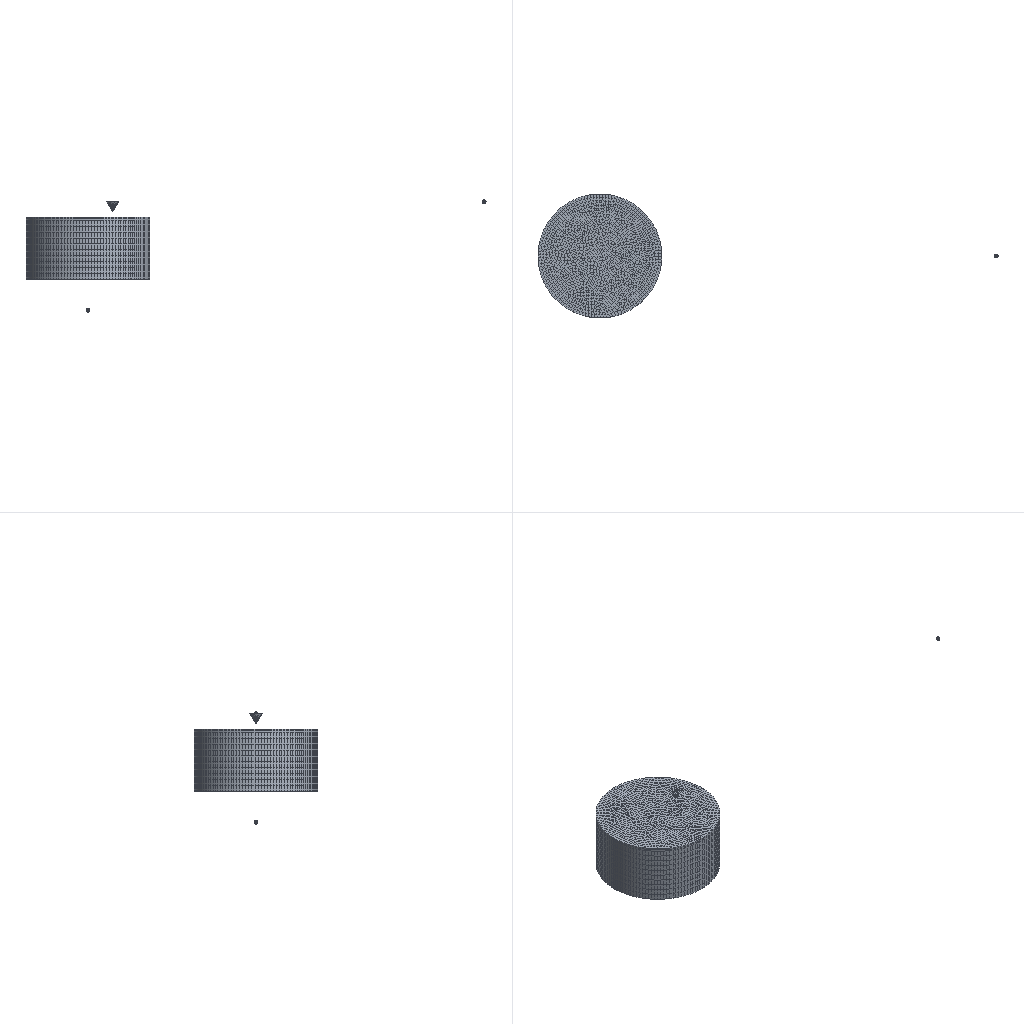Simulation study | abaqus
Set-up summary:
category,name,step,type,value,unit,region
solver,abaqus
solver,version,,,Abaqus/Explicit 2020
units,not stated in the deck,,not stated
analysis,deck,,transient,transient
load_step,Step-1,Step-1,transient
load_step,requested,,,1
mesh,nodes,,,27952
mesh,elements,,,30285
element_type,C3D4,,solid,8198
element_type,C3D8R,,solid,19488
element_type,C3D10M,,solid,2599
load,load commands in deck,,count,2
bc,support commands in deck,,count,7
material,TOOL,,in results
material,WORK,,in results
material,ZHONGJIAN,,in results
check,setup vs results,,match,"per instance, exact: element labels, types and connectivity; labels of the nodes the elements use; coordinates not compared"
Abaqus input file, long lists of numbers shortened:
*Heading
** Job name: Job-1 Model name: Model-1
** Generated by: Abaqus/CAE 2020
*Preprint, echo=NO, model=NO, history=NO, contact=NO
**
** PARTS
**
*Part, name=tool
*Node
      1, 0.07265, -0.0003314,           0.
      2,           0.,           0.,           0.
** (4216 more lines like these left out)
*Element, type=C3D10M
   1,  357,  358,  359,  360,  636,  635,  634,  638,  637,  639
   2,  357,  361,  362,  363,  642,  641,  640,  644,  643,  645
** (2597 more lines like these left out)
*Nset, nset=Set-1, generate
    1,  4218,     1
*Elset, elset=Set-1, generate
    1,  2599,     1
** Section: tool
*Solid Section, elset=Set-1, material=tool
,
*End Part
**
*Part, name=work
*Node
      1,    8.841,  -17.94,          19.
      2,   14.142,  -14.142,           0.
** (21942 more lines like these left out)
*Element, type=C3D8R
    1,    54,   669,   660,    53,  3554,  6614,  6605,  3553
    2,   579,  1605,   918,  1626,  6524,  7550,  6863,  7571
** (19486 more lines like these left out)
*Nset, nset=Set-1, generate
     1,  21944,      1
*Elset, elset=Set-1, generate
     1,  19488,      1
** Section: work
*Solid Section, elset=Set-1, material=work
,
*End Part
**
*Part, name=zhongjian
*Node
      1,  0.1247,  0.5869,           0.
      2,  0.244,  0.5481,           0.
** (892 more lines like these left out)
*Element, type=C3D4
   1, 390, 391, 392, 393
   2, 390, 394, 395, 393
** (4097 more lines like these left out)
*Node
    895,           0., -3.67394056e-17,           0.
*Nset, nset=zhongjian-RefPt_, internal
895,
*Nset, nset=Set-12, generate
   1,  894,    1
*Elset, elset=Set-12, generate
    1,  4099,     1
** Section: zhongjian
*Solid Section, elset=Set-12, material=ZHONGJIAN
,
*End Part
**
**
** ASSEMBLY
**
*Assembly, name=Assembly
**
*Instance, name=tool-1, part=tool
          8.,           0.,          22.
          8.,           0.,          22., 7.,           0.,          22., 90.
*End Instance
**
*Instance, name=work-1, part=work
*End Instance
**
*Instance, name=zhongjian-1, part=zhongjian
        128.,           0.,          25.
*End Instance
**
*Instance, name=zhongjian-2, part=zhongjian
          0.,           0.,         -10.
*End Instance
**
*Node
      1,           0.,           0.,          20.
*Node
      2,           8., -6.12323426e-17,          25.
*Nset, nset=O```
 2,
*Nset, nset=Set-2, instance=work-1
    2,  130,  131,  132,  133,  134,  135,  136,  137,  138,  139,  140,  141,  142,  143,  144
  145,  146,  147,  148,  149,  150,  151,  152,  153,  154,  155,  156,  157,  158,  159,  160
** (104 more lines like these left out)
*Elset, elset=Set-2, instance=work-1, generate
 14617,  16240,      1
*Nset, nset=Set-6, instance=zhongjian-1
 895,
*Nset, nset=Set-11, instance=zhongjian-1
 895,
*Nset, nset=Set-12, instance=zhongjian-1, generate
   1,  389,    1
*Elset, elset=Set-12, instance=zhongjian-1
    4,   92,  207,  218,  228,  238,  271,  289,  299,  351,  358,  363,  392,  402,  418,  434
  457,  464,  525,  530,  587,  619,  629,  652,  671,  724,  817,  883,  901,  938,  980, 1055
** (47 more lines like these left out)
*Nset, nset=Set-14, instance=zhongjian-1
   1,   2,   3,   4,   5,   6,   7,   8,   9,  10,  11,  12,  13,  14,  15,  16
  17,  18,  19,  20,  21,  22,  23,  24,  25,  26,  27,  28,  29,  30,  31,  32
** (23 more lines like these left out)
*Elset, elset=Set-14, instance=zhongjian-1
    4,   92,  207,  218,  228,  238,  271,  289,  299,  351,  358,  363,  392,  402,  418,  434
  457,  464,  525,  530,  587,  619,  629,  652,  671,  724,  817,  883,  901,  938,  980, 1055
** (47 more lines like these left out)
*Nset, nset=Set-15, instance=zhongjian-1
 895,
*Nset, nset=Set-20
 2,
*Nset, nset=Set-21
 2,
*Nset, nset=Set-23, instance=zhongjian-2
 895,
*Nset, nset=Set-24, instance=work-1
    2,  130,  131,  132,  133,  134,  135,  136,  137,  138,  139,  140,  141,  142,  143,  144
  145,  146,  147,  148,  149,  150,  151,  152,  153,  154,  155,  156,  157,  158,  159,  160
** (104 more lines like these left out)
*Elset, elset=Set-24, instance=work-1, generate
 14617,  16240,      1
*Nset, nset=Set-27, instance=zhongjian-1
 895,
*Nset, nset=b_Set-4, instance=tool-1, generate
    1,  4218,     1
*Elset, elset=b_Set-4, instance=tool-1, generate
    1,  2599,     1
*Nset, nset=m_Set-7, instance=zhongjian-1
 895,
*Nset, nset=m_Set-10
 2,
*Nset, nset=m_Set-13, instance=zhongjian-1
 895,
*Nset, nset=m_Set-22, instance=zhongjian-2
 895,
*Nset, nset=m_Set-25, instance=zhongjian-1
 895,
*Nset, nset=m_Set-31, instance=zhongjian-1
 895,
*Nset, nset=s_Set-9, instance=work-1
     1,     3,     4,     5,     6,     7,     8,     9,    10,    11,    12,    13,    14,    15,    16,    17
    18,    19,    20,    21,    22,    23,    24,    25,    26,    27,    28,    29,    30,    31,    32,    33
** (315 more lines like these left out)
*Elset, elset=s_Set-9, instance=work-1, generate
 16241,  19488,      1
*Nset, nset=s_Set-28, instance=zhongjian-1
 895,
*Nset, nset=s_Set-29, instance=zhongjian-1
 895,
*Nset, nset=s_Set-30, instance=zhongjian-1
 15,
*Nset, nset=_PickedSet18, internal
 2,
*Elset, elset=_m_Surf-3_S3, internal, instance=tool-1
   78,   91,   99,  120,  134,  140,  142,  156,  171,  174,  175,  227,  236,  300,  303,  334
  345,  361,  391,  438,  442,  466,  473,  545,  556,  563,  577,  583,  616,  617,  669,  683
** (35 more lines like these left out)
*Elset, elset=_m_Surf-3_S4, internal, instance=tool-1
  110,  555, 1022, 1034, 1139, 1517, 1537, 1685, 1759, 1847, 2324, 2399
*Elset, elset=_m_Surf-3_S1, internal, instance=tool-1
  346,  510,  736,  906,  960,  978, 1446, 1805, 2076, 2161, 2174, 2238, 2314, 2341, 2522
*Elset, elset=_m_Surf-3_S2, internal, instance=tool-1
  665,  757, 1449, 1497, 1588, 1601, 1647, 1705, 1760, 1790, 1821, 1831, 1834, 1878, 1899, 1962
 2052, 2064, 2112, 2437
*Surface, type=ELEMENT, name=m_Surf-3
_m_Surf-3_S3, S3
_m_Surf-3_S4, S4
_m_Surf-3_S2, S2
_m_Surf-3_S1, S1
*Elset, elset=_s_Surf-1_S3, internal, instance=tool-1
   78,   91,   99,  120,  134,  140,  142,  156,  171,  174,  175,  227,  236,  300,  303,  334
  345,  361,  391,  438,  442,  466,  473,  497,  545,  563,  577,  583,  617,  669,  683,  709
** (36 more lines like these left out)
*Elset, elset=_s_Surf-1_S4, internal, instance=tool-1
  110,  555,  583,  848,  887, 1022, 1034, 1139, 1430, 1455, 1469, 1511, 1517, 1537, 1569, 1610
 1638, 1685, 1719, 1847, 1857, 1877, 2324, 2399, 2425, 2508
*Elset, elset=_s_Surf-1_S1, internal, instance=tool-1
  346,  510,  736,  906,  960,  978, 1428, 1429, 1431, 1446, 1527, 1622, 1713, 1715, 1805, 1953
 2076, 2153, 2161, 2174, 2238, 2302, 2341, 2522
*Elset, elset=_s_Surf-1_S2, internal, instance=tool-1
  665,  757, 1164, 1363, 1446, 1449, 1497, 1521, 1574, 1588, 1601, 1634, 1639, 1643, 1646, 1647
 1697, 1705, 1714, 1760, 1762, 1788, 1790, 1821, 1831, 1834, 1878, 1899, 1962, 1970, 1982, 1995
** (1 more lines like these left out)
*Surface, type=ELEMENT, name=s_Surf-1
_s_Surf-1_S3, S3
_s_Surf-1_S4, S4
_s_Surf-1_S2, S2
_s_Surf-1_S1, S1
*Elset, elset=_s_Surf-2_S3, internal, instance=tool-1
   78,   91,   99,  120,  134,  140,  142,  156,  171,  174,  175,  227,  236,  300,  303,  334
  345,  361,  391,  438,  442,  466,  473,  497,  545,  563,  577,  583,  617,  669,  683,  709
** (36 more lines like these left out)
*Elset, elset=_s_Surf-2_S4, internal, instance=tool-1
  110,  555,  583,  848,  887, 1022, 1034, 1139, 1430, 1455, 1469, 1511, 1517, 1537, 1569, 1610
 1638, 1685, 1719, 1847, 1857, 1877, 2324, 2399, 2425, 2508
*Elset, elset=_s_Surf-2_S1, internal, instance=tool-1
  346,  510,  736,  906,  960,  978, 1428, 1429, 1431, 1446, 1527, 1622, 1713, 1715, 1805, 1953
 2076, 2153, 2161, 2174, 2238, 2302, 2341, 2522
*Elset, elset=_s_Surf-2_S2, internal, instance=tool-1
  665,  757, 1164, 1363, 1446, 1449, 1497, 1521, 1574, 1588, 1601, 1634, 1639, 1643, 1646, 1647
 1697, 1705, 1714, 1760, 1762, 1788, 1790, 1821, 1831, 1834, 1878, 1899, 1962, 1970, 1982, 1995
** (1 more lines like these left out)
*Surface, type=ELEMENT, name=s_Surf-2
_s_Surf-2_S3, S3
_s_Surf-2_S4, S4
_s_Surf-2_S2, S2
_s_Surf-2_S1, S1
*Elset, elset=_s_Surf-4_S3, internal, instance=tool-1
   78,   91,   99,  120,  134,  140,  142,  156,  171,  174,  175,  227,  236,  300,  303,  334
  345,  361,  391,  438,  442,  466,  473,  497,  545,  563,  577,  583,  617,  669,  683,  709
** (36 more lines like these left out)
*Elset, elset=_s_Surf-4_S4, internal, instance=tool-1
  110,  555,  583,  848,  887, 1022, 1034, 1139, 1430, 1455, 1469, 1511, 1517, 1537, 1569, 1610
 1638, 1685, 1719, 1847, 1857, 1877, 2324, 2399, 2425, 2508
*Elset, elset=_s_Surf-4_S1, internal, instance=tool-1
  346,  510,  736,  906,  960,  978, 1428, 1429, 1431, 1446, 1527, 1622, 1713, 1715, 1805, 1953
 2076, 2153, 2161, 2174, 2238, 2302, 2341, 2522
*Elset, elset=_s_Surf-4_S2, internal, instance=tool-1
  665,  757, 1164, 1363, 1446, 1449, 1497, 1521, 1574, 1588, 1601, 1634, 1639, 1643, 1646, 1647
 1697, 1705, 1714, 1760, 1762, 1788, 1790, 1821, 1831, 1834, 1878, 1899, 1962, 1970, 1982, 1995
** (1 more lines like these left out)
*Surface, type=ELEMENT, name=s_Surf-4
_s_Surf-4_S3, S3
_s_Surf-4_S4, S4
_s_Surf-4_S2, S2
_s_Surf-4_S1, S1
*Elset, elset=_s_Surf-5_S4, internal, instance=zhongjian-1
    4,  207,  619, 1283, 1533, 1714, 1784, 1867, 1928, 1998, 2148, 2163, 2289, 2383, 2459, 2481
 2483, 2546, 2592, 2733, 2800, 2803, 2851, 2913, 2943, 2958, 3155, 3221, 3281, 3352, 3359, 3364
** (1 more lines like these left out)
*Elset, elset=_s_Surf-5_S3, internal, instance=zhongjian-1
   92,  218,  228,  238,  289,  299,  351,  358,  363,  392,  402,  418,  434,  457,  464,  587
  671,  724,  817,  883,  938,  980, 1058, 1138, 1180, 1244, 1252, 1309, 1325, 1385, 1394, 1402
** (42 more lines like these left out)
*Elset, elset=_s_Surf-5_S1, internal, instance=zhongjian-1
  271,  525,  901, 1055, 1059, 1234, 1942, 2336, 2472, 2613, 2645, 2752, 3469, 3771, 3814
*Elset, elset=_s_Surf-5_S2, internal, instance=zhongjian-1
  530,  629,  652, 1859, 1898, 1899, 1979, 2210, 2256, 2330, 2343, 2370, 2910, 3041, 3271, 3345
 3375, 3392, 3471, 3618, 3844, 3951
*Surface, type=ELEMENT, name=s_Surf-5
_s_Surf-5_S4, S4
_s_Surf-5_S3, S3
_s_Surf-5_S2, S2
_s_Surf-5_S1, S1
*Elset, elset=_s_Surf-6_S3, internal, instance=tool-1
   78,   91,   99,  120,  134,  140,  142,  156,  171,  174,  175,  227,  236,  300,  303,  334
  345,  361,  391,  438,  442,  466,  473,  497,  545,  563,  577,  583,  617,  669,  683,  709
** (36 more lines like these left out)
*Elset, elset=_s_Surf-6_S4, internal, instance=tool-1
  110,  555,  583,  848,  887, 1022, 1034, 1139, 1430, 1455, 1469, 1511, 1517, 1537, 1569, 1610
 1638, 1685, 1719, 1847, 1857, 1877, 2324, 2399, 2425, 2508
*Elset, elset=_s_Surf-6_S1, internal, instance=tool-1
  346,  510,  736,  906,  960,  978, 1428, 1429, 1431, 1446, 1527, 1622, 1713, 1715, 1805, 1953
 2076, 2153, 2161, 2174, 2238, 2302, 2341, 2522
*Elset, elset=_s_Surf-6_S2, internal, instance=tool-1
  665,  757, 1164, 1363, 1446, 1449, 1497, 1521, 1574, 1588, 1601, 1634, 1639, 1643, 1646, 1647
 1697, 1705, 1714, 1760, 1762, 1788, 1790, 1821, 1831, 1834, 1878, 1899, 1962, 1970, 1982, 1995
** (1 more lines like these left out)
*Surface, type=ELEMENT, name=s_Surf-6
_s_Surf-6_S3, S3
_s_Surf-6_S4, S4
_s_Surf-6_S2, S2
_s_Surf-6_S1, S1
*Elset, elset=_s_Surf-7_S4, internal, instance=zhongjian-1
    4,  207,  619, 1283, 1533, 1714, 1784, 1867, 1928, 1998, 2148, 2163, 2289, 2383, 2459, 2481
 2483, 2546, 2592, 2733, 2800, 2803, 2851, 2913, 2943, 2958, 3155, 3221, 3281, 3352, 3359, 3364
** (1 more lines like these left out)
*Elset, elset=_s_Surf-7_S3, internal, instance=zhongjian-1
   92,  218,  228,  238,  289,  299,  351,  358,  363,  392,  402,  418,  434,  457,  464,  587
  671,  724,  817,  883,  938,  980, 1058, 1138, 1180, 1244, 1252, 1309, 1325, 1385, 1394, 1402
** (42 more lines like these left out)
*Elset, elset=_s_Surf-7_S1, internal, instance=zhongjian-1
  271,  525,  901, 1055, 1059, 1234, 1942, 2336, 2472, 2613, 2645, 2752, 3469, 3771, 3814
*Elset, elset=_s_Surf-7_S2, internal, instance=zhongjian-1
  530,  629,  652, 1859, 1898, 1899, 1979, 2210, 2256, 2330, 2343, 2370, 2910, 3041, 3271, 3345
 3375, 3392, 3471, 3618, 3844, 3951
*Surface, type=ELEMENT, name=s_Surf-7
_s_Surf-7_S4, S4
_s_Surf-7_S3, S3
_s_Surf-7_S2, S2
_s_Surf-7_S1, S1
*Elset, elset=_s_Surf-8_S3, internal, instance=tool-1
   78,   91,   99,  120,  134,  140,  142,  156,  171,  174,  175,  227,  236,  300,  303,  334
  345,  361,  391,  438,  442,  466,  473,  497,  545,  563,  577,  583,  617,  669,  683,  709
** (36 more lines like these left out)
*Elset, elset=_s_Surf-8_S4, internal, instance=tool-1
  110,  555,  583,  848,  887, 1022, 1034, 1139, 1430, 1455, 1469, 1511, 1517, 1537, 1569, 1610
 1638, 1685, 1719, 1847, 1857, 1877, 2324, 2399, 2425, 2508
*Elset, elset=_s_Surf-8_S1, internal, instance=tool-1
  346,  510,  736,  906,  960,  978, 1428, 1429, 1431, 1446, 1527, 1622, 1713, 1715, 1805, 1953
 2076, 2153, 2161, 2174, 2238, 2302, 2341, 2522
*Elset, elset=_s_Surf-8_S2, internal, instance=tool-1
  665,  757, 1164, 1363, 1446, 1449, 1497, 1521, 1574, 1588, 1601, 1634, 1639, 1643, 1646, 1647
 1697, 1705, 1714, 1760, 1762, 1788, 1790, 1821, 1831, 1834, 1878, 1899, 1962, 1970, 1982, 1995
** (1 more lines like these left out)
*Surface, type=ELEMENT, name=s_Surf-8
_s_Surf-8_S3, S3
_s_Surf-8_S4, S4
_s_Surf-8_S2, S2
_s_Surf-8_S1, S1
*Elset, elset=_s_Surf-9_S4, internal, instance=zhongjian-1
    4,  207,  619, 1283, 1533, 1714, 1784, 1867, 1928, 1998, 2148, 2163, 2289, 2383, 2459, 2481
 2483, 2546, 2592, 2733, 2800, 2803, 2851, 2913, 2943, 2958, 3155, 3221, 3281, 3352, 3359, 3364
** (1 more lines like these left out)
*Elset, elset=_s_Surf-9_S3, internal, instance=zhongjian-1
   92,  218,  228,  238,  289,  299,  351,  358,  363,  392,  402,  418,  434,  457,  464,  587
  671,  724,  817,  883,  938,  980, 1058, 1138, 1180, 1244, 1252, 1309, 1325, 1385, 1394, 1402
** (42 more lines like these left out)
*Elset, elset=_s_Surf-9_S1, internal, instance=zhongjian-1
  271,  525,  901, 1055, 1059, 1234, 1942, 2336, 2472, 2613, 2645, 2752, 3469, 3771, 3814
*Elset, elset=_s_Surf-9_S2, internal, instance=zhongjian-1
  530,  629,  652, 1859, 1898, 1899, 1979, 2210, 2256, 2330, 2343, 2370, 2910, 3041, 3271, 3345
 3375, 3392, 3471, 3618, 3844, 3951
*Surface, type=ELEMENT, name=s_Surf-9
_s_Surf-9_S4, S4
_s_Surf-9_S3, S3
_s_Surf-9_S2, S2
_s_Surf-9_S1, S1
*Elset, elset=_s_Surf-10_S3, internal, instance=tool-1
   78,   91,   99,  120,  134,  140,  142,  156,  171,  174,  175,  227,  236,  300,  303,  334
  345,  361,  391,  438,  442,  466,  473,  497,  545,  556,  563,  577,  583,  616,  617,  669
** (37 more lines like these left out)
*Elset, elset=_s_Surf-10_S4, internal, instance=tool-1
  110,  555,  583,  848,  887, 1022, 1034, 1139, 1430, 1455, 1469, 1511, 1517, 1537, 1569, 1610
 1638, 1685, 1719, 1759, 1847, 1857, 1877, 2324, 2399, 2425, 2508
*Elset, elset=_s_Surf-10_S1, internal, instance=tool-1
  346,  510,  736,  906,  960,  978, 1428, 1429, 1431, 1446, 1527, 1622, 1713, 1715, 1805, 1953
 2076, 2153, 2161, 2174, 2238, 2302, 2314, 2341, 2522
*Elset, elset=_s_Surf-10_S2, internal, instance=tool-1
  665,  757, 1164, 1363, 1446, 1449, 1497, 1521, 1574, 1588, 1601, 1634, 1639, 1643, 1646, 1647
 1697, 1705, 1714, 1760, 1762, 1788, 1790, 1821, 1831, 1834, 1878, 1899, 1962, 1970, 1982, 1995
** (1 more lines like these left out)
*Surface, type=ELEMENT, name=s_Surf-10
_s_Surf-10_S3, S3
_s_Surf-10_S4, S4
_s_Surf-10_S2, S2
_s_Surf-10_S1, S1
*Elset, elset=_s_Surf-11_S4, internal, instance=zhongjian-1
    4,  207,  619, 1283, 1533, 1714, 1784, 1867, 1928, 1998, 2148, 2163, 2289, 2383, 2459, 2481
 2483, 2546, 2592, 2733, 2800, 2803, 2851, 2913, 2943, 2958, 3155, 3221, 3281, 3352, 3359, 3364
** (1 more lines like these left out)
*Elset, elset=_s_Surf-11_S3, internal, instance=zhongjian-1
   92,  218,  228,  238,  289,  299,  351,  358,  363,  392,  402,  418,  434,  457,  464,  587
  671,  724,  817,  883,  938,  980, 1058, 1138, 1180, 1244, 1252, 1309, 1325, 1385, 1394, 1402
** (42 more lines like these left out)
*Elset, elset=_s_Surf-11_S1, internal, instance=zhongjian-1
  271,  525,  901, 1055, 1059, 1234, 1942, 2336, 2472, 2613, 2645, 2752, 3469, 3771, 3814
*Elset, elset=_s_Surf-11_S2, internal, instance=zhongjian-1
  530,  629,  652, 1859, 1898, 1899, 1979, 2210, 2256, 2330, 2343, 2370, 2910, 3041, 3271, 3345
 3375, 3392, 3471, 3618, 3844, 3951
*Surface, type=ELEMENT, name=s_Surf-11
_s_Surf-11_S4, S4
_s_Surf-11_S3, S3
_s_Surf-11_S2, S2
_s_Surf-11_S1, S1
*Surface, type=NODE, name=s_Set-9_CNS_, internal
s_Set-9, 1.
** Constraint: Constraint-4
*Coupling, constraint name=Constraint-4, ref node=m_Set-31, surface=s_Surf-11
*Kinematic
** Constraint: drive-tool
*Coupling, constraint name=drive-tool, ref node=m_Set-25, surface=s_Surf-10
*Kinematic
** Constraint: rigid
*Rigid Body, ref node=_PickedSet18, elset=b_Set-4
*End Assembly
**
** MATERIALS
**
*Material, name=ZHONGJIAN
*Density
 2.4e-09,
*Elastic
200000., 0.25
*Material, name=tool
*Density
 3.48e-09,
*Elastic
700000., 0.29
*Material, name=work
*Damage Initiation, criterion=JOHNSON COOK
 0.1,  0.76,  1.57, 0.005, -0.84, 1500.,   20.,    1.
*Damage Evolution, type=DISPLACEMENT
 0.01,
*Density
 7.85e-09,
*Elastic
210000., 0.31
*Plastic, hardening=JOHNSON COOK
507.,  320., 0.064,  1.06, 1500.,   20.
*Rate Dependent, type=JOHNSON COOK
 0.28,1.
**
** INTERACTION PROPERTIES
**
*Surface Interaction, name=IntProp-1
*Friction
 0.3,
*Surface Behavior, pressure-overclosure=HARD
** ----------------------------------------------------------------
**
** STEP: Step-1
**
*Step, name=Step-1, nlgeom=YES
*Dynamic, Explicit
, 0.5
*Bulk Viscosity
0.06, 1.2
** Mass Scaling: Semi-Automatic
**               Whole Model
*Fixed Mass Scaling, dt=1e-05, type=below min
**
** BOUNDARY CONDITIONS
**
** Name: BC-2 Type: 对称/反对称/完全固定
*Boundary
Set-24, ENCASTRE
** Name: drive-tool Type: speed/angular velocity
*Boundary, type=VELOCITY
Set-27, 1, 1
Set-27, 2, 2
Set-27, 3, 3, -5.
Set-27, 4, 4
Set-27, 5, 5
Set-27, 6, 6, 119.
**
** INTERACTIONS
**
** Interaction: Int-1
*Contact Pair, interaction=IntProp-1, mechanical constraint=PENALTY, cpset=Int-1
m_Surf-3, s_Set-9_CNS_
**
** OUTPUT REQUESTS
**
*Restart, write, number interval=1, time marks=NO
**
** FIELD OUTPUT: F-Output-1
**
*Output, field, number interval=200
*Node Output
A, AR, AT, RF, U, V
*Element Output, directions=YES
E, LE, MISES, PE, PEEQ, PEEQVAVG, PEVAVG, S, STATUS, SVAVG
*Contact Output
CSTRESS,
**
** HISTORY OUTPUT: H-Output-1
**
*Output, history, variable=PRESELECT
*End Step
Results summary:
result,step,Step-1,completed,increments=42287 time=0.5/0.5
result,analysis,,,transient
result,last_loadstep,,,1
result,primary field,,,U
result,reaction total,,FX,14.451,model units
result,reaction total,,FY,-3.626,model units
result,reaction total,,FZ,17.32,model units